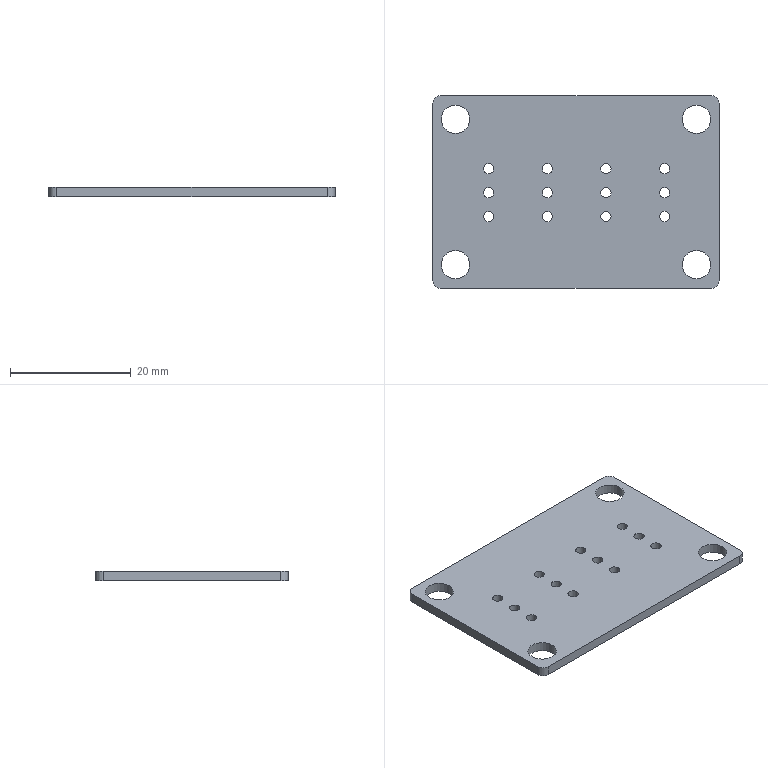Part | STEP file | SOLID | 1 solid | 26 faces | box 47.38 x 31.85 x 1.6 mm | volume 2258 mm3 | cylinder 20 | plane 6 | commonest cylinder face diameters 1.7 x12 2.54 x4 4.7 x4